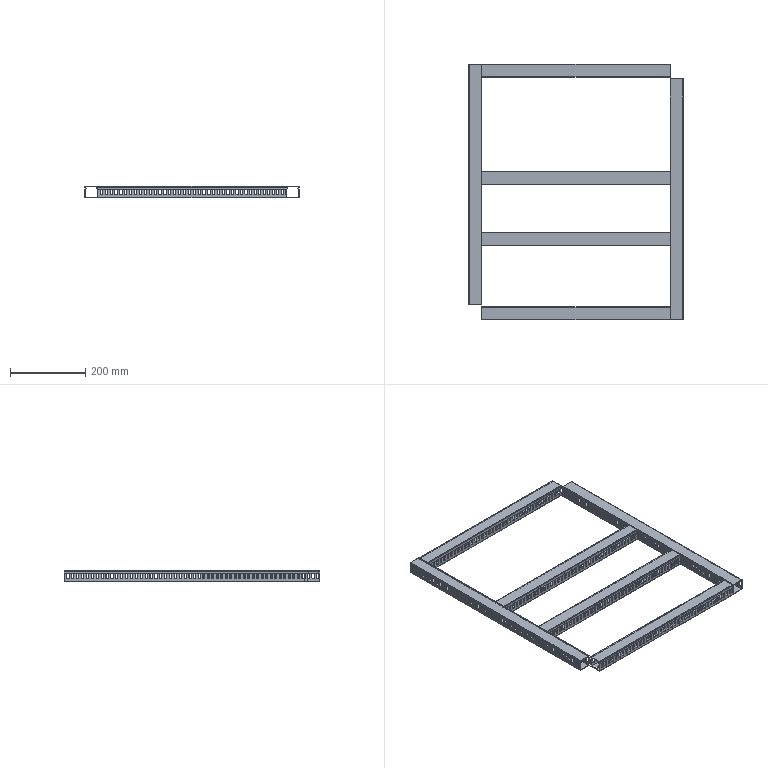Part | SolidWorks | 12 solids | 4648 faces | volume 575981 mm3 | plane 3944 | cylinder 704 | commonest cylinder face diameters 6 x524 5 x132 1 x24 0.2 x12 2 x12